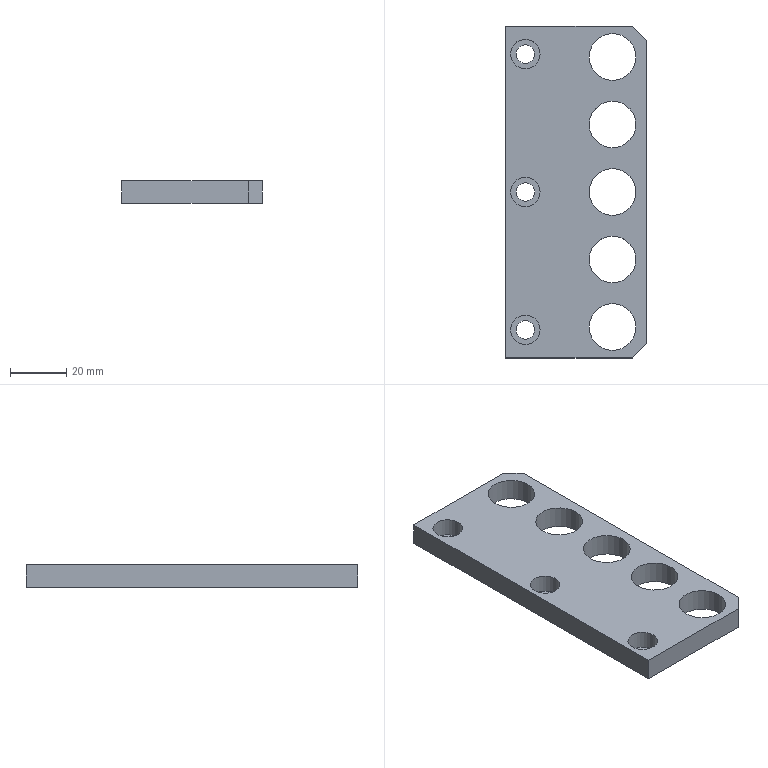CAM job | NX | 3-axis milling, drilling | part box 50 x 118 x 8 mm | stock box 57 x 128 x 12 mm
Tools:
number,name,description,diameter,corner_radius,flute_length,length,flutes
5,D4点钻,定心钻D4,4.0,0.0,43.0,75.0,2
2,D6点钻,定心钻D6,6.0,0.0,57.0,93.0,2
6,D6精光,D6,6.0,0.0,16.0,60.0,2
4,D8开粗,D8,8.0,0.0,20.0,60.0,2
1,D63R0.8,方肩铣刀片,63.0,0.8,15.0,80.0,2
3,Z6.5,Z6.5直柄钻头,6.5,0.0,63.0,101.0,2
Operations:
program,operation,operation_type,tool,method,geometry_group,spindle_rpm,surface_speed,feed_per_tooth,feed_cut,feed_plunge,cut_length_mm,path_length_mm,cut_time_min,machine_time_min
XX-CNC1,PLANAR_MILL,PlanarMilling,D63R0.8,METHOD,W1,2500.0,494.0,0.16,800.0,100.0,196.0,252.0,0.245,0.2506
XX-CNC1,DRILLING,Operation,D6点钻,METHOD,MCS_1,2000.0,37.0,0.0375,150.0,0.0,36.0,379.091,0.24,0.2743
XX-CNC1,DRILLING_COPY,Operation,Z6.5,METHOD,MCS_1,2000.0,40.0,0.0375,150.0,0.0,120.0,547.091,0.8,0.8427
XX-CNC1,ADAPTIVE_MILLING,CavityMilling,D8开粗,METHOD,W1,3500.0,87.0,0.2143,1500.0,100.0,10658.43,12792.194,6.778,6.992
XX-CNC1,PLANAR_MILL_1,PlanarMilling,D8开粗,METHOD,W1,3500.0,87.0,0.2143,1500.0,100.0,671.27,963.264,0.4475,0.4767
XX-CNC1,PLANAR_MILL_2,PlanarMilling,D4点钻,METHOD,W1,3000.0,37.0,0.1333,800.0,100.0,344.511,402.511,0.4306,0.4364
XX-CNC1,PLANAR_MILL_2_COPY,PlanarMilling,D4点钻,METHOD,W1,3000.0,37.0,0.1333,800.0,100.0,284.671,654.671,0.3558,0.3928
XX-CNC1,PLANAR_MILL_2_COPY_COPY,PlanarMilling,D4点钻,METHOD,W1,3000.0,37.0,0.1333,800.0,100.0,102.481,372.87,0.1281,0.1551
XX-CNC1,PLANAR_MILL_3,PlanarMilling,D6精光,METHOD,MCS_1,3500.0,65.0,0.1143,800.0,100.0,356.279,430.279,0.4453,0.4527
XX-CNC1,PLANAR_MILL_4,PlanarMilling,D6精光,METHOD,MCS_1,3500.0,65.0,0.1143,800.0,100.0,224.672,674.672,0.2808,0.3258
XX-CNC1,PLANAR_MILL_5,PlanarMilling,D6精光,METHOD,MCS_1,3500.0,65.0,0.1143,800.0,100.0,85.261,390.264,0.1066,0.1371
XX-CNC2,PLANAR_MILL_6,PlanarMilling,D63R0.8,METHOD,MCS_2,2500.0,100.0,0.1178,800.0,100.0,2625.598,5679.972,3.282,3.587
XX-CNC2,PLANAR_MILL_6_COPY,PlanarMilling,D63R0.8,METHOD,MCS_2,2500.0,100.0,0.1178,800.0,100.0,202.0,258.0,0.2525,0.2581
XX-CNC2,PLANAR_MILL_7,PlanarMilling,D4点钻,METHOD,MCS_2,3000.0,100.0,0.1178,800.0,100.0,346.511,402.511,0.4331,0.4387
XX-CNC2,PLANAR_MILL_8,PlanarMilling,D4点钻,METHOD,MCS_2,3000.0,100.0,0.1178,800.0,100.0,333.438,1015.211,0.4168,0.485